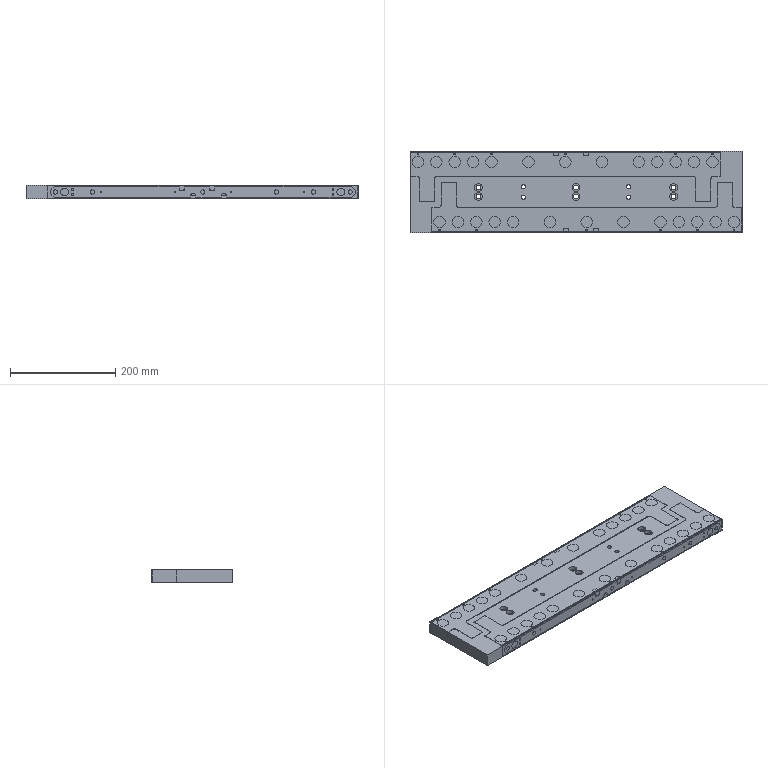NC program | NX | posted with a generic post | part box 631 x 154 x 25 mm
Lines 18142 to 18383 of 18383:
(ZLEVEL_PROFILE_COPY_1_COPY_COPY_COPY_COPY_2 , TOOL : D6A45)
N36252 T07 M6
N36254 G54
N36256 G17 G0 G90 X-129.422 Y55.574 B0. C0. S7000 M3
N36258 G43 Z30. H7
N36260 Z-1.2
N36262 G94 G1 X-129.98 Y56.541 F1000.
N36264 G3 X-130.5 Y56.841 R0.6
N36266 X-140.341 Y47. R9.841
N36268 X-130.5 Y56.841 R-9.841
N36270 X-131.02 Y56.541 R0.6
N36272 G1 X-131.578 Y55.574
N36274 G0 Z30.
N36276 X-164.422
N36278 Z-1.2
N36280 G1 X-164.98 Y56.541
N36282 G3 X-165.5 Y56.841 R0.6
N36284 X-175.341 Y47. R9.841
N36286 X-165.5 Y56.841 R-9.841
N36288 X-166.02 Y56.541 R0.6
N36290 G1 X-166.578 Y55.574
N36292 G0 Z30.
N36294 X-209.074 Y48.078
N36296 Z-1.2
N36298 G1 X-210.041 Y47.52
N36300 G3 X-210.341 Y47. R0.6
N36302 X-200.5 Y37.159 R9.841
N36304 X-210.341 Y47. R-9.841
N36306 X-210.041 Y46.48 R0.6
N36308 G1 X-209.074 Y45.922
N36310 G0 Z30.
N36312 X-94.422 Y55.574
N36314 Z-1.2
N36316 G1 X-94.98 Y56.541
N36318 G3 X-95.5 Y56.841 R0.6
N36320 X-105.341 Y47. R9.841
N36322 X-95.5 Y56.841 R-9.841
N36324 X-96.02 Y56.541 R0.6
N36326 G1 X-96.578 Y55.574
N36328 G0 Z30.
N36330 X325.578
N36332 Z-1.2
N36334 G1 X325.02 Y56.541
N36336 G3 X324.5 Y56.841 R0.6
N36338 X314.659 Y47. R9.841
N36340 X324.5 Y56.841 R-9.841
N36342 X323.98 Y56.541 R0.6
N36344 G1 X323.422 Y55.574
N36346 G0 Z30.
N36348 X10.578
N36350 Z-1.2
N36352 G1 X10.02 Y56.541
N36354 G3 X9.5 Y56.841 R0.6
N36356 X-0.341 Y47. R9.841
N36358 X9.5 Y56.841 R-9.841
N36360 X8.98 Y56.541 R0.6
N36362 G1 X8.422 Y55.574
N36364 G0 Z30.
N36366 X360.578
N36368 Z-1.2
N36370 G1 X360.02 Y56.541
N36372 G3 X359.5 Y56.841 R0.6
N36374 X349.659 Y47. R9.841
N36376 X359.5 Y56.841 R-9.841
N36378 X358.98 Y56.541 R0.6
N36380 G1 X358.422 Y55.574
N36382 G0 Z30.
N36384 X290.578
N36386 Z-1.2
N36388 G1 X290.02 Y56.541
N36390 G3 X289.5 Y56.841 R0.6
N36392 X279.659 Y47. R9.841
N36394 X289.5 Y56.841 R-9.841
N36396 X288.98 Y56.541 R0.6
N36398 G1 X288.422 Y55.574
N36400 G0 Z30.
N36402 X255.578
N36404 Z-1.2
N36406 G1 X255.02 Y56.541
N36408 G3 X254.5 Y56.841 R0.6
N36410 X244.659 Y47. R9.841
N36412 X254.5 Y56.841 R-9.841
N36414 X253.98 Y56.541 R0.6
N36416 G1 X253.422 Y55.574
N36418 G0 Z30.
N36420 X220.578
N36422 Z-1.2
N36424 G1 X220.02 Y56.541
N36426 G3 X219.5 Y56.841 R0.6
N36428 X209.659 Y47. R9.841
N36430 X219.5 Y56.841 R-9.841
N36432 X218.98 Y56.541 R0.6
N36434 G1 X218.422 Y55.574
N36436 G0 Z30.
N36438 X150.578
N36440 Z-1.2
N36442 G1 X150.02 Y56.541
N36444 G3 X149.5 Y56.841 R0.6
N36446 X139.659 Y47. R9.841
N36448 X149.5 Y56.841 R-9.841
N36450 X148.98 Y56.541 R0.6
N36452 G1 X148.422 Y55.574
N36454 G0 Z30.
N36456 X80.578
N36458 Z-1.2
N36460 G1 X80.02 Y56.541
N36462 G3 X79.5 Y56.841 R0.6
N36464 X69.659 Y47. R9.841
N36466 X79.5 Y56.841 R-9.841
N36468 X78.98 Y56.541 R0.6
N36470 G1 X78.422 Y55.574
N36472 G0 Z30.
N36474 X-59.422
N36476 Z-1.2
N36478 G1 X-59.98 Y56.541
N36480 G3 X-60.5 Y56.841 R0.6
N36482 X-70.341 Y47. R9.841
N36484 X-60.5 Y56.841 R-9.841
N36486 X-61.02 Y56.541 R0.6
N36488 G1 X-61.578 Y55.574
N36490 G0 Z30.
N36492 X409.074 Y-68.078
N36494 Z-1.2
N36496 G1 X410.041 Y-67.52
N36498 G3 X410.341 Y-67. R0.6
N36500 X400.5 Y-57.159 R9.841
N36502 X410.341 Y-67. R-9.841
N36504 X410.041 Y-66.48 R0.6
N36506 G1 X409.074 Y-65.922
N36508 G0 Z30.
N36510 X364.422 Y-75.574
N36512 Z-1.2
N36514 G1 X364.98 Y-76.541
N36516 G3 X365.5 Y-76.841 R0.6
N36518 X375.341 Y-67. R9.841
N36520 X365.5 Y-76.841 R-9.841
N36522 X366.02 Y-76.541 R0.6
N36524 G1 X366.578 Y-75.574
N36526 G0 Z30.
N36528 X329.422
N36530 Z-1.2
N36532 G1 X329.98 Y-76.541
N36534 G3 X330.5 Y-76.841 R0.6
N36536 X340.341 Y-67. R9.841
N36538 X330.5 Y-76.841 R-9.841
N36540 X331.02 Y-76.541 R0.6
N36542 G1 X331.578 Y-75.574
N36544 G0 Z30.
N36546 X294.422
N36548 Z-1.2
N36550 G1 X294.98 Y-76.541
N36552 G3 X295.5 Y-76.841 R0.6
N36554 X305.341 Y-67. R9.841
N36556 X295.5 Y-76.841 R-9.841
N36558 X296.02 Y-76.541 R0.6
N36560 G1 X296.578 Y-75.574
N36562 G0 Z30.
N36564 X259.422
N36566 Z-1.2
N36568 G1 X259.98 Y-76.541
N36570 G3 X260.5 Y-76.841 R0.6
N36572 X270.341 Y-67. R9.841
N36574 X260.5 Y-76.841 R-9.841
N36576 X261.02 Y-76.541 R0.6
N36578 G1 X261.578 Y-75.574
N36580 G0 Z30.
N36582 X189.422
N36584 Z-1.2
N36586 G1 X189.98 Y-76.541
N36588 G3 X190.5 Y-76.841 R0.6
N36590 X200.341 Y-67. R9.841
N36592 X190.5 Y-76.841 R-9.841
N36594 X191.02 Y-76.541 R0.6
N36596 G1 X191.578 Y-75.574
N36598 G0 Z30.
N36600 X119.422
N36602 Z-1.2
N36604 G1 X119.98 Y-76.541
N36606 G3 X120.5 Y-76.841 R0.6
N36608 X130.341 Y-67. R9.841
N36610 X120.5 Y-76.841 R-9.841
N36612 X121.02 Y-76.541 R0.6
N36614 G1 X121.578 Y-75.574
N36616 G0 Z30.
N36618 X49.422
N36620 Z-1.2
N36622 G1 X49.98 Y-76.541
N36624 G3 X50.5 Y-76.841 R0.6
N36626 X60.341 Y-67. R9.841
N36628 X50.5 Y-76.841 R-9.841
N36630 X51.02 Y-76.541 R0.6
N36632 G1 X51.578 Y-75.574
N36634 G0 Z30.
N36636 X-20.578
N36638 Z-1.2
N36640 G1 X-20.02 Y-76.541
N36642 G3 X-19.5 Y-76.841 R0.6
N36644 X-9.659 Y-67. R9.841
N36646 X-19.5 Y-76.841 R-9.841
N36648 X-18.98 Y-76.541 R0.6
N36650 G1 X-18.422 Y-75.574
N36652 G0 Z30.
N36654 X-55.578
N36656 Z-1.2
N36658 G1 X-55.02 Y-76.541
N36660 G3 X-54.5 Y-76.841 R0.6
N36662 X-44.659 Y-67. R9.841
N36664 X-54.5 Y-76.841 R-9.841
N36666 X-53.98 Y-76.541 R0.6
N36668 G1 X-53.422 Y-75.574
N36670 G0 Z30.
N36672 X-90.578
N36674 Z-1.2
N36676 G1 X-90.02 Y-76.541
N36678 G3 X-89.5 Y-76.841 R0.6
N36680 X-79.659 Y-67. R9.841
N36682 X-89.5 Y-76.841 R-9.841
N36684 X-88.98 Y-76.541 R0.6
N36686 G1 X-88.422 Y-75.574
N36688 G0 Z30.
N36690 X-125.578
N36692 Z-1.2
N36694 G1 X-125.02 Y-76.541
N36696 G3 X-124.5 Y-76.841 R0.6
N36698 X-114.659 Y-67. R9.841
N36700 X-124.5 Y-76.841 R-9.841
N36702 X-123.98 Y-76.541 R0.6
N36704 G1 X-123.422 Y-75.574
N36706 G0 Z30.
N36708 X-160.578
N36710 Z-1.2
N36712 G1 X-160.02 Y-76.541
N36714 G3 X-159.5 Y-76.841 R0.6
N36716 X-149.659 Y-67. R9.841
N36718 X-159.5 Y-76.841 R-9.841
N36720 X-158.98 Y-76.541 R0.6
N36722 G1 X-158.422 Y-75.574
N36724 G0 Z30.
N36726 M5
N36728 M2